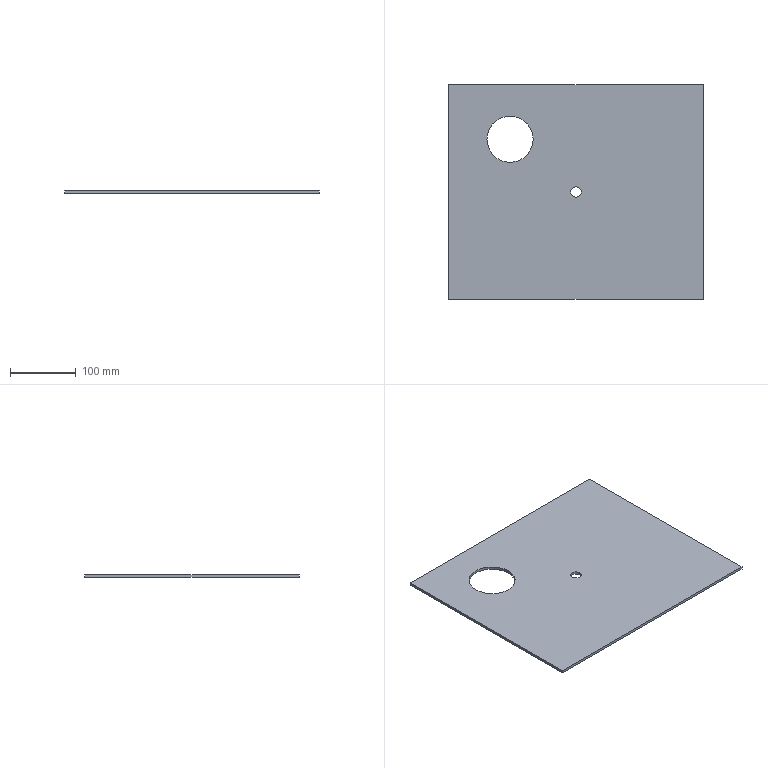Part | SolidWorks | features Extrusion 1, ICE 1 | 1 solid | 10 faces | box 386 x 326 x 4 mm | volume 487146 mm3 | plane 6 | cylinder 4 | commonest cylinder face diameters 16 x2 70 x2
STEP:
#1=CARTESIAN_POINT('',(-8.,0.,-2.));
#2=VERTEX_POINT('',#1);
#3=CARTESIAN_POINT('',(8.,0.,-2.));
#4=VERTEX_POINT('',#3);
#5=CARTESIAN_POINT('',(0.,0.,-2.));
#6=DIRECTION('',(0.,0.,1.));
#7=DIRECTION('',(1.,0.,0.));
#8=AXIS2_PLACEMENT_3D('',#5,#6,#7);
#9=CIRCLE('',#8,8.);
#10=EDGE_CURVE('',#2,#4,#9,.T.);
#11=ORIENTED_EDGE('',*,*,#10,.F.);
#12=CARTESIAN_POINT('',(-8.,0.,2.));
#13=VERTEX_POINT('',#12);
#14=CARTESIAN_POINT('',(-8.,0.,-12.));
#15=DIRECTION('',(0.,0.,1.));
#16=VECTOR('',#15,1000.);
#17=LINE('',#14,#16);
#18=EDGE_CURVE('',#2,#13,#17,.T.);
#19=ORIENTED_EDGE('',*,*,#18,.T.);
#20=CARTESIAN_POINT('',(8.,0.,2.));
#21=VERTEX_POINT('',#20);
#22=CARTESIAN_POINT('',(0.,0.,2.));
#23=DIRECTION('',(0.,0.,1.));
#24=DIRECTION('',(1.,0.,0.));
#25=AXIS2_PLACEMENT_3D('',#22,#23,#24);
#26=CIRCLE('',#25,8.);
#27=EDGE_CURVE('',#13,#21,#26,.T.);
#28=ORIENTED_EDGE('',*,*,#27,.T.);
#29=CARTESIAN_POINT('',(8.,0.,-12.));
#30=DIRECTION('',(0.,0.,1.));
#31=VECTOR('',#30,1000.);
#32=LINE('',#29,#31);
#33=EDGE_CURVE('',#4,#21,#32,.T.);
#34=ORIENTED_EDGE('',*,*,#33,.F.);
#35=EDGE_LOOP('',(#11,#19,#28,#34));
#36=FACE_OUTER_BOUND('',#35,.T.);
#37=CARTESIAN_POINT('',(0.,0.,-12.));
#38=DIRECTION('',(0.,0.,1.));
#39=DIRECTION('',(1.,0.,0.));
#40=AXIS2_PLACEMENT_3D('',#37,#38,#39);
#41=CYLINDRICAL_SURFACE('',#40,8.);
#42=ADVANCED_FACE('',(#36),#41,.F.);
#43=CARTESIAN_POINT('',(-135.,80.,-2.));
#44=VERTEX_POINT('',#43);
#45=CARTESIAN_POINT('',(-65.,80.,-2.));
#46=VERTEX_POINT('',#45);
#47=CARTESIAN_POINT('',(-100.,80.,-2.));
#48=DIRECTION('',(0.,0.,1.));
#49=DIRECTION('',(1.,0.,0.));
#50=AXIS2_PLACEMENT_3D('',#47,#48,#49);
#51=CIRCLE('',#50,35.);
#52=EDGE_CURVE('',#44,#46,#51,.T.);
#53=ORIENTED_EDGE('',*,*,#52,.F.);
#54=CARTESIAN_POINT('',(-135.,80.,2.));
#55=VERTEX_POINT('',#54);
#56=CARTESIAN_POINT('',(-135.,80.,-12.));
#57=DIRECTION('',(0.,0.,1.));
#58=VECTOR('',#57,1000.);
#59=LINE('',#56,#58);
#60=EDGE_CURVE('',#44,#55,#59,.T.);
#61=ORIENTED_EDGE('',*,*,#60,.T.);
#62=CARTESIAN_POINT('',(-65.,80.,2.));
#63=VERTEX_POINT('',#62);
#64=CARTESIAN_POINT('',(-100.,80.,2.));
#65=DIRECTION('',(0.,0.,1.));
#66=DIRECTION('',(1.,0.,0.));
#67=AXIS2_PLACEMENT_3D('',#64,#65,#66);
#68=CIRCLE('',#67,35.);
#69=EDGE_CURVE('',#55,#63,#68,.T.);
#70=ORIENTED_EDGE('',*,*,#69,.T.);
#71=CARTESIAN_POINT('',(-65.,80.,-12.));
#72=DIRECTION('',(0.,0.,1.));
#73=VECTOR('',#72,1000.);
#74=LINE('',#71,#73);
#75=EDGE_CURVE('',#46,#63,#74,.T.);
#76=ORIENTED_EDGE('',*,*,#75,.F.);
#77=EDGE_LOOP('',(#53,#61,#70,#76));
#78=FACE_OUTER_BOUND('',#77,.T.);
#79=CARTESIAN_POINT('',(-100.,80.,-12.));
#80=DIRECTION('',(0.,0.,1.));
#81=DIRECTION('',(1.,0.,0.));
#82=AXIS2_PLACEMENT_3D('',#79,#80,#81);
#83=CYLINDRICAL_SURFACE('',#82,35.);
#84=ADVANCED_FACE('',(#78),#83,.F.);
#85=CARTESIAN_POINT('',(-193.,163.,2.));
#86=VERTEX_POINT('',#85);
#87=CARTESIAN_POINT('',(-193.,-163.,2.));
#88=VERTEX_POINT('',#87);
#89=CARTESIAN_POINT('',(-193.,163.,2.));
#90=DIRECTION('',(0.,-1.,0.));
#91=VECTOR('',#90,1000.);
#92=LINE('',#89,#91);
#93=EDGE_CURVE('',#86,#88,#92,.T.);
#94=ORIENTED_EDGE('',*,*,#93,.F.);
#95=CARTESIAN_POINT('',(-193.,163.,-2.));
#96=VERTEX_POINT('',#95);
#97=CARTESIAN_POINT('',(-193.,163.,-2.));
#98=DIRECTION('',(0.,0.,1.));
#99=VECTOR('',#98,1000.);
#100=LINE('',#97,#99);
#101=EDGE_CURVE('',#96,#86,#100,.T.);
#102=ORIENTED_EDGE('',*,*,#101,.F.);
#103=CARTESIAN_POINT('',(-193.,-163.,-2.));
#104=VERTEX_POINT('',#103);
#105=CARTESIAN_POINT('',(-193.,163.,-2.));
#106=DIRECTION('',(0.,-1.,0.));
#107=VECTOR('',#106,1000.);
#108=LINE('',#105,#107);
#109=EDGE_CURVE('',#96,#104,#108,.T.);
#110=ORIENTED_EDGE('',*,*,#109,.T.);
#111=CARTESIAN_POINT('',(-193.,-163.,-2.));
#112=DIRECTION('',(0.,0.,1.));
#113=VECTOR('',#112,1000.);
#114=LINE('',#111,#113);
#115=EDGE_CURVE('',#104,#88,#114,.T.);
#116=ORIENTED_EDGE('',*,*,#115,.T.);
#117=EDGE_LOOP('',(#94,#102,#110,#116));
#118=FACE_OUTER_BOUND('',#117,.T.);
#119=CARTESIAN_POINT('',(-193.,163.,-2.));
#120=DIRECTION('',(-1.,0.,0.));
#121=DIRECTION('',(0.,0.,1.));
#122=AXIS2_PLACEMENT_3D('',#119,#120,#121);
#123=PLANE('',#122);
#124=ADVANCED_FACE('',(#118),#123,.T.);
#125=CARTESIAN_POINT('',(193.,163.,2.));
#126=VERTEX_POINT('',#125);
#127=CARTESIAN_POINT('',(193.,163.,2.));
#128=DIRECTION('',(-1.,0.,0.));
#129=VECTOR('',#128,1000.);
#130=LINE('',#127,#129);
#131=EDGE_CURVE('',#126,#86,#130,.T.);
#132=ORIENTED_EDGE('',*,*,#131,.F.);
#133=CARTESIAN_POINT('',(193.,163.,-2.));
#134=VERTEX_POINT('',#133);
#135=CARTESIAN_POINT('',(193.,163.,-2.));
#136=DIRECTION('',(0.,0.,1.));
#137=VECTOR('',#136,1000.);
#138=LINE('',#135,#137);
#139=EDGE_CURVE('',#134,#126,#138,.T.);
#140=ORIENTED_EDGE('',*,*,#139,.F.);
#141=CARTESIAN_POINT('',(193.,163.,-2.));
#142=DIRECTION('',(-1.,0.,0.));
#143=VECTOR('',#142,1000.);
#144=LINE('',#141,#143);
#145=EDGE_CURVE('',#134,#96,#144,.T.);
#146=ORIENTED_EDGE('',*,*,#145,.T.);
#147=ORIENTED_EDGE('',*,*,#101,.T.);
#148=EDGE_LOOP('',(#132,#140,#146,#147));
#149=FACE_OUTER_BOUND('',#148,.T.);
#150=CARTESIAN_POINT('',(193.,163.,-2.));
#151=DIRECTION('',(0.,1.,0.));
#152=DIRECTION('',(0.,0.,1.));
#153=AXIS2_PLACEMENT_3D('',#150,#151,#152);
#154=PLANE('',#153);
#155=ADVANCED_FACE('',(#149),#154,.T.);
#156=CARTESIAN_POINT('',(193.,-163.,2.));
#157=VERTEX_POINT('',#156);
#158=CARTESIAN_POINT('',(193.,-163.,2.));
#159=DIRECTION('',(0.,1.,0.));
#160=VECTOR('',#159,1000.);
#161=LINE('',#158,#160);
#162=EDGE_CURVE('',#157,#126,#161,.T.);
#163=ORIENTED_EDGE('',*,*,#162,.F.);
#164=CARTESIAN_POINT('',(193.,-163.,-2.));
#165=VERTEX_POINT('',#164);
#166=CARTESIAN_POINT('',(193.,-163.,-2.));
#167=DIRECTION('',(0.,0.,1.));
#168=VECTOR('',#167,1000.);
#169=LINE('',#166,#168);
#170=EDGE_CURVE('',#165,#157,#169,.T.);
#171=ORIENTED_EDGE('',*,*,#170,.F.);
#172=CARTESIAN_POINT('',(193.,-163.,-2.));
#173=DIRECTION('',(0.,1.,0.));
#174=VECTOR('',#173,1000.);
#175=LINE('',#172,#174);
#176=EDGE_CURVE('',#165,#134,#175,.T.);
#177=ORIENTED_EDGE('',*,*,#176,.T.);
#178=ORIENTED_EDGE('',*,*,#139,.T.);
#179=EDGE_LOOP('',(#163,#171,#177,#178));
#180=FACE_OUTER_BOUND('',#179,.T.);
#181=CARTESIAN_POINT('',(193.,-163.,-2.));
#182=DIRECTION('',(1.,0.,0.));
#183=DIRECTION('',(0.,0.,-1.));
#184=AXIS2_PLACEMENT_3D('',#181,#182,#183);
#185=PLANE('',#184);
#186=ADVANCED_FACE('',(#180),#185,.T.);
#187=CARTESIAN_POINT('',(-193.,-163.,2.));
#188=DIRECTION('',(1.,0.,0.));
#189=VECTOR('',#188,1000.);
#190=LINE('',#187,#189);
#191=EDGE_CURVE('',#88,#157,#190,.T.);
#192=ORIENTED_EDGE('',*,*,#191,.F.);
#193=ORIENTED_EDGE('',*,*,#115,.F.);
#194=CARTESIAN_POINT('',(-193.,-163.,-2.));
#195=DIRECTION('',(1.,0.,0.));
#196=VECTOR('',#195,1000.);
#197=LINE('',#194,#196);
#198=EDGE_CURVE('',#104,#165,#197,.T.);
#199=ORIENTED_EDGE('',*,*,#198,.T.);
#200=ORIENTED_EDGE('',*,*,#170,.T.);
#201=EDGE_LOOP('',(#192,#193,#199,#200));
#202=FACE_OUTER_BOUND('',#201,.T.);
#203=CARTESIAN_POINT('',(-193.,-163.,-2.));
#204=DIRECTION('',(0.,-1.,0.));
#205=DIRECTION('',(0.,0.,-1.));
#206=AXIS2_PLACEMENT_3D('',#203,#204,#205);
#207=PLANE('',#206);
#208=ADVANCED_FACE('',(#202),#207,.T.);
#209=CARTESIAN_POINT('',(0.,0.,-2.));
#210=DIRECTION('',(0.,0.,1.));
#211=DIRECTION('',(1.,0.,0.));
#212=AXIS2_PLACEMENT_3D('',#209,#210,#211);
#213=CIRCLE('',#212,8.);
#214=EDGE_CURVE('',#4,#2,#213,.T.);
#215=ORIENTED_EDGE('',*,*,#214,.T.);
#216=ORIENTED_EDGE('',*,*,#10,.T.);
#217=EDGE_LOOP('',(#215,#216));
#218=FACE_BOUND('',#217,.T.);
#219=CARTESIAN_POINT('',(-100.,80.,-2.));
#220=DIRECTION('',(0.,0.,1.));
#221=DIRECTION('',(1.,0.,0.));
#222=AXIS2_PLACEMENT_3D('',#219,#220,#221);
#223=CIRCLE('',#222,35.);
#224=EDGE_CURVE('',#46,#44,#223,.T.);
#225=ORIENTED_EDGE('',*,*,#224,.T.);
#226=ORIENTED_EDGE('',*,*,#52,.T.);
#227=EDGE_LOOP('',(#225,#226));
#228=FACE_BOUND('',#227,.T.);
#229=ORIENTED_EDGE('',*,*,#109,.F.);
#230=ORIENTED_EDGE('',*,*,#145,.F.);
#231=ORIENTED_EDGE('',*,*,#176,.F.);
#232=ORIENTED_EDGE('',*,*,#198,.F.);
#233=EDGE_LOOP('',(#229,#230,#231,#232));
#234=FACE_OUTER_BOUND('',#233,.T.);
#235=CARTESIAN_POINT('',(0.,0.,-2.));
#236=DIRECTION('',(0.,0.,1.));
#237=DIRECTION('',(1.,0.,0.));
#238=AXIS2_PLACEMENT_3D('',#235,#236,#237);
#239=PLANE('',#238);
#240=ADVANCED_FACE('',(#218,#228,#234),#239,.F.);
#241=CARTESIAN_POINT('',(0.,0.,2.));
#242=DIRECTION('',(0.,0.,1.));
#243=DIRECTION('',(1.,0.,0.));
#244=AXIS2_PLACEMENT_3D('',#241,#242,#243);
#245=CIRCLE('',#244,8.);
#246=EDGE_CURVE('',#21,#13,#245,.T.);
#247=ORIENTED_EDGE('',*,*,#246,.F.);
#248=ORIENTED_EDGE('',*,*,#27,.F.);
#249=EDGE_LOOP('',(#247,#248));
#250=FACE_BOUND('',#249,.T.);
#251=CARTESIAN_POINT('',(-100.,80.,2.));
#252=DIRECTION('',(0.,0.,1.));
#253=DIRECTION('',(1.,0.,0.));
#254=AXIS2_PLACEMENT_3D('',#251,#252,#253);
#255=CIRCLE('',#254,35.);
#256=EDGE_CURVE('',#63,#55,#255,.T.);
#257=ORIENTED_EDGE('',*,*,#256,.F.);
#258=ORIENTED_EDGE('',*,*,#69,.F.);
#259=EDGE_LOOP('',(#257,#258));
#260=FACE_BOUND('',#259,.T.);
#261=ORIENTED_EDGE('',*,*,#93,.T.);
#262=ORIENTED_EDGE('',*,*,#191,.T.);
#263=ORIENTED_EDGE('',*,*,#162,.T.);
#264=ORIENTED_EDGE('',*,*,#131,.T.);
#265=EDGE_LOOP('',(#261,#262,#263,#264));
#266=FACE_OUTER_BOUND('',#265,.T.);
#267=CARTESIAN_POINT('',(0.,0.,2.));
#268=DIRECTION('',(0.,0.,1.));
#269=DIRECTION('',(1.,0.,0.));
#270=AXIS2_PLACEMENT_3D('',#267,#268,#269);
#271=PLANE('',#270);
#272=ADVANCED_FACE('',(#250,#260,#266),#271,.T.);
#273=ORIENTED_EDGE('',*,*,#60,.F.);
#274=ORIENTED_EDGE('',*,*,#224,.F.);
#275=ORIENTED_EDGE('',*,*,#75,.T.);
#276=ORIENTED_EDGE('',*,*,#256,.T.);
#277=EDGE_LOOP('',(#273,#274,#275,#276));
#278=FACE_OUTER_BOUND('',#277,.T.);
#279=CARTESIAN_POINT('',(-100.,80.,-12.));
#280=DIRECTION('',(0.,0.,1.));
#281=DIRECTION('',(1.,0.,0.));
#282=AXIS2_PLACEMENT_3D('',#279,#280,#281);
#283=CYLINDRICAL_SURFACE('',#282,35.);
#284=ADVANCED_FACE('',(#278),#283,.F.);
#285=ORIENTED_EDGE('',*,*,#18,.F.);
#286=ORIENTED_EDGE('',*,*,#214,.F.);
#287=ORIENTED_EDGE('',*,*,#33,.T.);
#288=ORIENTED_EDGE('',*,*,#246,.T.);
#289=EDGE_LOOP('',(#285,#286,#287,#288));
#290=FACE_OUTER_BOUND('',#289,.T.);
#291=CARTESIAN_POINT('',(0.,0.,-12.));
#292=DIRECTION('',(0.,0.,1.));
#293=DIRECTION('',(1.,0.,0.));
#294=AXIS2_PLACEMENT_3D('',#291,#292,#293);
#295=CYLINDRICAL_SURFACE('',#294,8.);
#296=ADVANCED_FACE('',(#290),#295,.F.);
#297=CLOSED_SHELL('',(#42,#84,#124,#155,#186,#208,#240,#272,#284,#296));
#298=MANIFOLD_SOLID_BREP('',#297);
#299=CARTESIAN_POINT('',(0.,0.,0.));
#300=DIRECTION('',(0.,0.,1.));
#301=DIRECTION('',(1.,0.,0.));
#302=AXIS2_PLACEMENT_3D('',#299,#300,#301);
#303=(LENGTH_UNIT()NAMED_UNIT(*)SI_UNIT(.MILLI.,.METRE.));
#304=UNCERTAINTY_MEASURE_WITH_UNIT(LENGTH_MEASURE(0.00001),#303,'','');
#305=(NAMED_UNIT(*)PLANE_ANGLE_UNIT()SI_UNIT($,.RADIAN.));
#306=(NAMED_UNIT(*)SI_UNIT($,.STERADIAN.)SOLID_ANGLE_UNIT());
#307=(GEOMETRIC_REPRESENTATION_CONTEXT(3)GLOBAL_UNCERTAINTY_ASSIGNED_CONTEXT((#304))GLOBAL_UNIT_ASSIGNED_CONTEXT((#303,#305,#306))REPRESENTATION_CONTEXT('',''));
#308=ADVANCED_BREP_SHAPE_REPRESENTATION('',(#298,#302),#307);